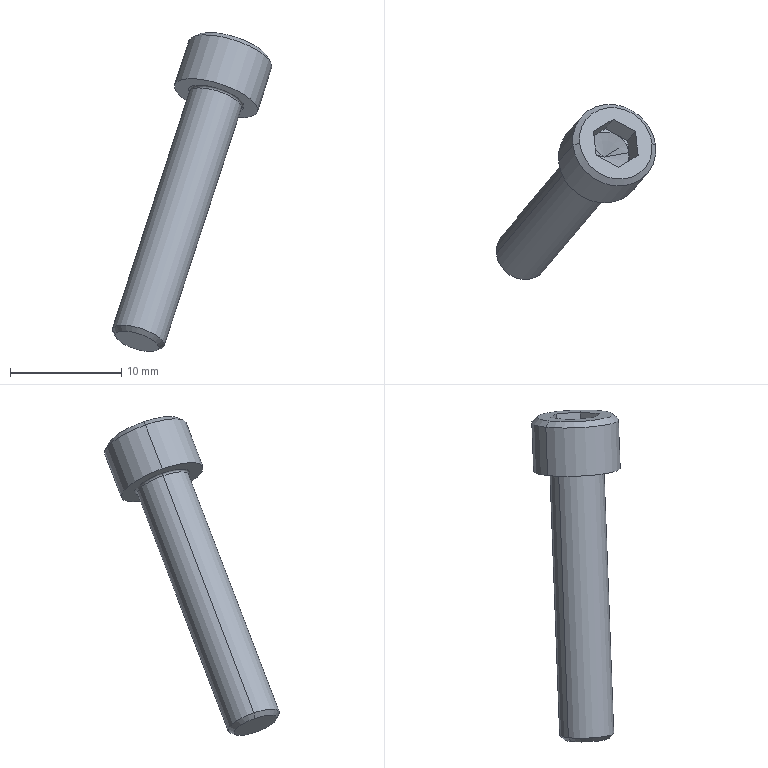Part | STEP file | 1 solid | 27 faces | box 14.373 x 15.735 x 28.731 mm | volume 656.353 mm3 | plane 15 | cone 6 | cylinder 4 | torus 2 | commonest cylinder face diameters 4.9 x2 7.84 x2